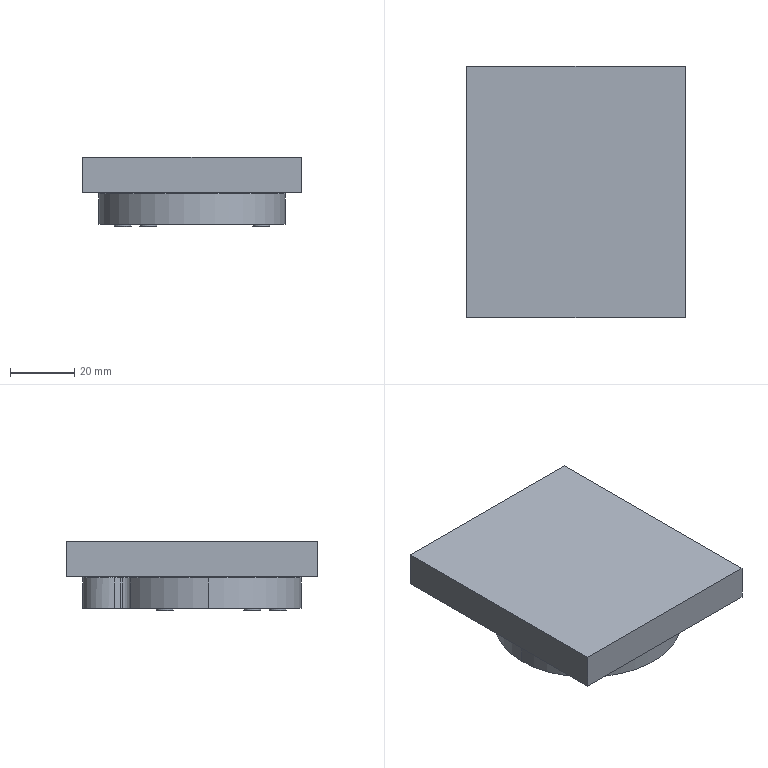NC program | NX | posted with a generic post | part box 68 x 78.27 x 21.8 mm
Lines 1195 to 2039 of 3502:
(ZLEVEL_PROFILE_1 , TOOL : D4)
N2376 T11 M6
N2378 G54
N2380 G17 G0 G90 X-5.374 Y-5.654 S9500 M3
N2382 G43 Z30. H11
N2384 Z1.5
N2386 G94 G1 X-5.297 Y-6.222 Z1.47 F1000.
N2388 X-5.21 Y-6.543 Z1.453
N2390 X-5.125 Y-6.859 Z1.435
N2392 X-4.841 Y-7.546 Z1.396
N2394 X-4.464 Y-8.186 Z1.358
N2396 X-4.003 Y-8.768 Z1.319
N2398 X-3.768 Y-8.996 Z1.301
N2400 X-3.75 Y-9.035 Z1.299
N2402 X3.732 Z0.907
N2404 X3.969 Y-8.808 Z0.89
N2406 X4.539 Y-8.078 Z0.841
N2408 X4.975 Y-7.261 Z0.793
N2410 X5.265 Y-6.382 Z0.744
N2412 X5.4 Y-5.466 Z0.696
N2414 Y-5.137 Z0.679
N2416 Y-4.808 Z0.661
N2418 X5.265 Y-3.892 Z0.613
N2420 X4.976 Y-3.012 Z0.564
N2422 X4.541 Y-2.194 Z0.516
N2424 X3.972 Y-1.462 Z0.467
N2426 X3.735 Y-1.235 Z0.45
N2428 X-3.735 Y-1.236 Z0.058
N2430 X-4.07 Y-1.588 Z0.033
N2432 X-4.287 Y-1.837 Z0.016
N2434 X-4.771 Y-2.589 Z-0.031
N2436 X-5.126 Y-3.411 Z-0.078
N2438 X-5.212 Y-3.729 Z-0.096
N2440 X-5.297 Y-4.047 Z-0.113
N2442 X-5.395 Y-4.77 Z-0.151
N2444 Y-5.499 Z-0.189
N2446 X-5.297 Y-6.222 Z-0.227
N2448 X-5.21 Y-6.543 Z-0.245
N2450 X-5.125 Y-6.859 Z-0.262
N2452 X-4.841 Y-7.546 Z-0.301
N2454 X-4.464 Y-8.186 Z-0.34
N2456 X-4.003 Y-8.768 Z-0.379
N2458 X-3.768 Y-8.996 Z-0.396
N2460 X-3.75 Y-9.035 Z-0.398
N2462 X-3.717 Z-0.4
N2464 X3.732 F2500.
N2466 G3 X5.4 Y-5.137 R5.389
N2468 X3.735 Y-1.235 R5.405
N2470 G1 X-3.735 Y-1.236
N2472 X-4.07 Y-1.588
N2474 G3 X-5.212 Y-3.729 R5.451
N2476 X-5.21 Y-6.543 R5.408
N2478 X-3.768 Y-8.996 R5.347
N2480 G1 X-3.765 Y-9.003
N2482 X-3.76 Y-9.027
N2484 X-3.74 Y-9.04
N2486 X-3.717 Y-9.035
N2488 X0.008 Z-0.446
N2490 X1.87 Z-0.469
N2492 X3.731 Y-9.034 Z-0.492
N2494 X3.79 Y-8.974 Z-0.493
N2496 X4.155 Y-8.579 Z-0.5
N2498 X4.252 Y-8.457 Z-0.502
N2500 X4.348 Y-8.335 Z-0.504
N2502 X4.439 Y-8.209 Z-0.506
N2504 X4.524 Y-8.078 Z-0.507
N2506 X4.609 Y-7.948 Z-0.509
N2508 X4.688 Y-7.814 Z-0.511
N2510 X4.762 Y-7.677 Z-0.513
N2512 X4.835 Y-7.539 Z-0.515
N2514 X4.966 Y-7.257 Z-0.519
N2516 X5.078 Y-6.967 Z-0.523
N2518 X5.129 Y-6.82 Z-0.525
N2520 X5.177 Y-6.672 Z-0.527
N2522 X5.217 Y-6.522 Z-0.529
N2524 X5.254 Y-6.37 Z-0.531
N2526 X5.318 Y-6.066 Z-0.534
N2528 X5.361 Y-5.758 Z-0.538
N2530 X5.385 Y-5.448 Z-0.542
N2532 X5.399 Y-5.137 Z-0.546
N2534 X5.385 Y-4.826 Z-0.55
N2536 X5.362 Y-4.516 Z-0.554
N2538 X5.318 Y-4.208 Z-0.557
N2540 X5.255 Y-3.903 Z-0.561
N2542 X5.218 Y-3.752 Z-0.563
N2544 X5.178 Y-3.601 Z-0.565
N2546 X5.13 Y-3.453 Z-0.567
N2548 X5.079 Y-3.306 Z-0.569
N2550 X5.025 Y-3.16 Z-0.571
N2552 X4.967 Y-3.016 Z-0.573
N2554 X4.902 Y-2.874 Z-0.575
N2556 X4.836 Y-2.733 Z-0.577
N2558 X4.689 Y-2.458 Z-0.581
N2560 X4.526 Y-2.194 Z-0.584
N2562 X4.44 Y-2.063 Z-0.586
N2564 X4.35 Y-1.937 Z-0.588
N2566 X4.253 Y-1.815 Z-0.59
N2568 X4.156 Y-1.693 Z-0.592
N2570 X3.734 Y-1.237 Z-0.6
N2572 X1.867 Y-1.235 Z-0.623
N2574 X0. Z-0.646
N2576 X-1.865 Z-0.669
N2578 X-3.728 Y-1.237 Z-0.692
N2580 X-3.777 Y-1.283 Z-0.693
N2582 X-4.07 Y-1.587 Z-0.698
N2584 X-4.26 Y-1.827 Z-0.702
N2586 X-4.444 Y-2.072 Z-0.706
N2588 X-4.609 Y-2.329 Z-0.709
N2590 X-4.762 Y-2.594 Z-0.713
N2592 X-4.831 Y-2.731 Z-0.715
N2594 X-4.9 Y-2.867 Z-0.717
N2596 X-4.962 Y-3.007 Z-0.719
N2598 X-5.018 Y-3.15 Z-0.721
N2600 X-5.073 Y-3.292 Z-0.723
N2602 X-5.125 Y-3.436 Z-0.725
N2604 X-5.17 Y-3.582 Z-0.727
N2606 X-5.212 Y-3.73 Z-0.728
N2608 X-5.281 Y-4.005 Z-0.732
N2610 X-5.331 Y-4.285 Z-0.735
N2612 X-5.37 Y-4.567 Z-0.739
N2614 X-5.392 Y-4.85 Z-0.742
N2616 X-5.4 Y-5.134 Z-0.746
N2618 X-5.393 Y-5.419 Z-0.749
N2620 X-5.37 Y-5.702 Z-0.753
N2622 X-5.331 Y-5.984 Z-0.757
N2624 X-5.28 Y-6.266 Z-0.76
N2626 X-5.21 Y-6.543 Z-0.764
N2628 X-5.172 Y-6.682 Z-0.765
N2630 X-5.13 Y-6.82 Z-0.767
N2632 X-5.082 Y-6.956 Z-0.769
N2634 X-5.03 Y-7.09 Z-0.771
N2636 X-4.977 Y-7.224 Z-0.772
N2638 X-4.922 Y-7.357 Z-0.774
N2640 X-4.857 Y-7.486 Z-0.776
N2642 X-4.792 Y-7.614 Z-0.778
N2644 X-4.727 Y-7.743 Z-0.78
N2646 X-4.656 Y-7.868 Z-0.781
N2648 X-4.578 Y-7.989 Z-0.783
N2650 X-4.501 Y-8.11 Z-0.785
N2652 X-4.336 Y-8.346 Z-0.789
N2654 X-4.158 Y-8.573 Z-0.792
N2656 X-3.966 Y-8.791 Z-0.796
N2658 X-3.742 Y-9.023 Z-0.8
N2660 X-3.717 Y-9.035
N2662 X0.009 Z-0.846
N2664 X1.871 Z-0.869
N2666 X3.732 Y-9.033 Z-0.892
N2668 X3.76 Y-9.006 Z-0.893
N2670 X3.974 Y-8.785 Z-0.896
N2672 X4.176 Y-8.552 Z-0.9
N2674 X4.272 Y-8.431 Z-0.902
N2676 X4.368 Y-8.31 Z-0.904
N2678 X4.455 Y-8.184 Z-0.906
N2680 X4.54 Y-8.055 Z-0.908
N2682 X4.701 Y-7.792 Z-0.912
N2684 X4.845 Y-7.519 Z-0.915
N2686 X4.973 Y-7.239 Z-0.919
N2688 X5.084 Y-6.951 Z-0.923
N2690 X5.134 Y-6.805 Z-0.925
N2692 X5.181 Y-6.658 Z-0.927
N2694 X5.221 Y-6.509 Z-0.929
N2696 X5.257 Y-6.359 Z-0.931
N2698 X5.318 Y-6.057 Z-0.934
N2700 X5.362 Y-5.752 Z-0.938
N2702 X5.385 Y-5.445 Z-0.942
N2704 X5.399 Y-5.137 Z-0.946
N2706 X5.385 Y-4.826 Z-0.95
N2708 X5.362 Y-4.516 Z-0.954
N2710 X5.318 Y-4.208 Z-0.957
N2712 X5.255 Y-3.903 Z-0.961
N2714 X5.218 Y-3.752 Z-0.963
N2716 X5.178 Y-3.601 Z-0.965
N2718 X5.13 Y-3.453 Z-0.967
N2720 X5.079 Y-3.306 Z-0.969
N2722 X4.967 Y-3.016 Z-0.973
N2724 X4.836 Y-2.733 Z-0.977
N2726 X4.689 Y-2.458 Z-0.981
N2728 X4.526 Y-2.194 Z-0.984
N2730 X4.441 Y-2.063 Z-0.986
N2732 X4.35 Y-1.937 Z-0.988
N2734 X4.253 Y-1.815 Z-0.99
N2736 X4.156 Y-1.693 Z-0.992
N2738 X3.734 Y-1.237 Z-1.
N2740 X1.867 Y-1.235 Z-1.023
N2742 X0. Z-1.046
N2744 X-1.867 Z-1.069
N2746 X-3.734 Y-1.238 Z-1.092
N2748 X-3.791 Y-1.297 Z-1.093
N2750 X-4.155 Y-1.693 Z-1.1
N2752 X-4.347 Y-1.938 Z-1.104
N2754 X-4.523 Y-2.194 Z-1.107
N2756 X-4.607 Y-2.326 Z-1.109
N2758 X-4.689 Y-2.457 Z-1.111
N2760 X-4.761 Y-2.595 Z-1.113
N2762 X-4.833 Y-2.734 Z-1.115
N2764 X-4.965 Y-3.015 Z-1.119
N2766 X-5.079 Y-3.305 Z-1.123
N2768 X-5.174 Y-3.601 Z-1.127
N2770 X-5.257 Y-3.901 Z-1.131
N2772 X-5.317 Y-4.206 Z-1.134
N2774 X-5.363 Y-4.514 Z-1.138
N2776 X-5.39 Y-4.824 Z-1.142
N2778 X-5.4 Y-5.135 Z-1.146
N2780 X-5.39 Y-5.446 Z-1.15
N2782 X-5.363 Y-5.756 Z-1.154
N2784 X-5.317 Y-6.064 Z-1.157
N2786 X-5.257 Y-6.369 Z-1.161
N2788 X-5.174 Y-6.669 Z-1.165
N2790 X-5.079 Y-6.965 Z-1.169
N2792 X-4.965 Y-7.254 Z-1.173
N2794 X-4.833 Y-7.536 Z-1.177
N2796 X-4.761 Y-7.674 Z-1.179
N2798 X-4.689 Y-7.812 Z-1.181
N2800 X-4.607 Y-7.944 Z-1.182
N2802 X-4.523 Y-8.075 Z-1.184
N2804 X-4.347 Y-8.332 Z-1.188
N2806 X-4.155 Y-8.576 Z-1.192
N2808 X-3.786 Y-8.978 Z-1.199
N2810 X-3.734 Y-9.032 Z-1.2
N2812 X-3.717 Y-9.035
N2814 X0.009 Z-1.246
N2816 X1.871 Z-1.269
N2818 X3.732 Y-9.033 Z-1.292
N2820 X3.76 Y-9.006 Z-1.293
N2822 X3.974 Y-8.785 Z-1.296
N2824 X4.176 Y-8.552 Z-1.3
N2826 X4.272 Y-8.431 Z-1.302
N2828 X4.368 Y-8.31 Z-1.304
N2830 X4.455 Y-8.184 Z-1.306
N2832 X4.54 Y-8.055 Z-1.308
N2834 X4.701 Y-7.792 Z-1.312
N2836 X4.845 Y-7.519 Z-1.315
N2838 X4.973 Y-7.239 Z-1.319
N2840 X5.084 Y-6.951 Z-1.323
N2842 X5.134 Y-6.805 Z-1.325
N2844 X5.181 Y-6.658 Z-1.327
N2846 X5.221 Y-6.509 Z-1.329
N2848 X5.257 Y-6.359 Z-1.331
N2850 X5.318 Y-6.057 Z-1.334
N2852 X5.362 Y-5.752 Z-1.338
N2854 X5.385 Y-5.445 Z-1.342
N2856 X5.399 Y-5.137 Z-1.346
N2858 X5.385 Y-4.826 Z-1.35
N2860 X5.362 Y-4.516 Z-1.354
N2862 X5.318 Y-4.208 Z-1.357
N2864 X5.255 Y-3.903 Z-1.361
N2866 X5.218 Y-3.752 Z-1.363
N2868 X5.178 Y-3.601 Z-1.365
N2870 X5.13 Y-3.453 Z-1.367
N2872 X5.079 Y-3.306 Z-1.369
N2874 X4.967 Y-3.016 Z-1.373
N2876 X4.836 Y-2.733 Z-1.377
N2878 X4.689 Y-2.458 Z-1.381
N2880 X4.526 Y-2.194 Z-1.384
N2882 X4.44 Y-2.063 Z-1.386
N2884 X4.35 Y-1.937 Z-1.388
N2886 X4.253 Y-1.815 Z-1.39
N2888 X4.156 Y-1.693 Z-1.392
N2890 X3.734 Y-1.237 Z-1.4
N2892 X1.867 Y-1.235 Z-1.423
N2894 X0. Z-1.446
N2896 X-1.867 Z-1.469
N2898 X-3.734 Y-1.238 Z-1.492
N2900 X-3.791 Y-1.297 Z-1.493
N2902 X-4.155 Y-1.693 Z-1.5
N2904 X-4.347 Y-1.938 Z-1.504
N2906 X-4.523 Y-2.194 Z-1.507
N2908 X-4.607 Y-2.326 Z-1.509
N2910 X-4.689 Y-2.457 Z-1.511
N2912 X-4.761 Y-2.595 Z-1.513
N2914 X-4.833 Y-2.734 Z-1.515
N2916 X-4.965 Y-3.015 Z-1.519
N2918 X-5.079 Y-3.305 Z-1.523
N2920 X-5.174 Y-3.601 Z-1.527
N2922 X-5.257 Y-3.901 Z-1.531
N2924 X-5.317 Y-4.206 Z-1.534
N2926 X-5.363 Y-4.514 Z-1.538
N2928 X-5.39 Y-4.824 Z-1.542
N2930 X-5.4 Y-5.135 Z-1.546
N2932 X-5.39 Y-5.446 Z-1.55
N2934 X-5.363 Y-5.756 Z-1.554
N2936 X-5.317 Y-6.064 Z-1.557
N2938 X-5.257 Y-6.369 Z-1.561
N2940 X-5.174 Y-6.669 Z-1.565
N2942 X-5.079 Y-6.965 Z-1.569
N2944 X-4.965 Y-7.254 Z-1.573
N2946 X-4.833 Y-7.536 Z-1.577
N2948 X-4.761 Y-7.674 Z-1.579
N2950 X-4.689 Y-7.812 Z-1.581
N2952 X-4.607 Y-7.944 Z-1.582
N2954 X-4.523 Y-8.075 Z-1.584
N2956 X-4.347 Y-8.332 Z-1.588
N2958 X-4.155 Y-8.576 Z-1.592
N2960 X-3.786 Y-8.978 Z-1.599
N2962 X-3.734 Y-9.031 Z-1.6
N2964 X-3.717 Y-9.035
N2966 X0.009 Z-1.646
N2968 X1.871 Z-1.669
N2970 X3.732 Y-9.033 Z-1.692
N2972 X3.76 Y-9.006 Z-1.693
N2974 X3.974 Y-8.785 Z-1.696
N2976 X4.176 Y-8.552 Z-1.7
N2978 X4.272 Y-8.431 Z-1.702
N2980 X4.368 Y-8.31 Z-1.704
N2982 X4.455 Y-8.184 Z-1.706
N2984 X4.54 Y-8.055 Z-1.708
N2986 X4.701 Y-7.792 Z-1.712
N2988 X4.845 Y-7.519 Z-1.715
N2990 X4.973 Y-7.239 Z-1.719
N2992 X5.084 Y-6.951 Z-1.723
N2994 X5.134 Y-6.805 Z-1.725
N2996 X5.181 Y-6.658 Z-1.727
N2998 X5.221 Y-6.509 Z-1.729
N3000 X5.257 Y-6.359 Z-1.731
N3002 X5.318 Y-6.057 Z-1.734
N3004 X5.362 Y-5.752 Z-1.738
N3006 X5.385 Y-5.445 Z-1.742
N3008 X5.399 Y-5.137 Z-1.746
N3010 X5.385 Y-4.826 Z-1.75
N3012 X5.362 Y-4.516 Z-1.754
N3014 X5.318 Y-4.208 Z-1.757
N3016 X5.255 Y-3.903 Z-1.761
N3018 X5.218 Y-3.752 Z-1.763
N3020 X5.178 Y-3.601 Z-1.765
N3022 X5.13 Y-3.453 Z-1.767
N3024 X5.079 Y-3.306 Z-1.769
N3026 X4.967 Y-3.016 Z-1.773
N3028 X4.836 Y-2.733 Z-1.777
N3030 X4.689 Y-2.458 Z-1.781
N3032 X4.526 Y-2.194 Z-1.784
N3034 X4.44 Y-2.063 Z-1.786
N3036 X4.35 Y-1.937 Z-1.788
N3038 X4.253 Y-1.815 Z-1.79
N3040 X4.156 Y-1.693 Z-1.792
N3042 X3.734 Y-1.237 Z-1.8
N3044 X1.867 Y-1.235 Z-1.823
N3046 X0. Z-1.846
N3048 X-1.867 Z-1.869
N3050 X-3.734 Y-1.238 Z-1.892
N3052 X-3.791 Y-1.297 Z-1.893
N3054 X-4.155 Y-1.693 Z-1.9
N3056 X-4.347 Y-1.938 Z-1.904
N3058 X-4.523 Y-2.194 Z-1.907
N3060 X-4.607 Y-2.326 Z-1.909
N3062 X-4.689 Y-2.457 Z-1.911
N3064 X-4.761 Y-2.595 Z-1.913
N3066 X-4.833 Y-2.734 Z-1.915
N3068 X-4.965 Y-3.015 Z-1.919
N3070 X-5.079 Y-3.305 Z-1.923
N3072 X-5.174 Y-3.601 Z-1.927
N3074 X-5.257 Y-3.901 Z-1.931
N3076 X-5.317 Y-4.206 Z-1.934
N3078 X-5.363 Y-4.514 Z-1.938
N3080 X-5.39 Y-4.824 Z-1.942
N3082 X-5.4 Y-5.135 Z-1.946
N3084 X-5.39 Y-5.446 Z-1.95
N3086 X-5.363 Y-5.756 Z-1.954
N3088 X-5.317 Y-6.064 Z-1.957
N3090 X-5.257 Y-6.369 Z-1.961
N3092 X-5.174 Y-6.669 Z-1.965
N3094 X-5.079 Y-6.965 Z-1.969
N3096 X-4.965 Y-7.254 Z-1.973
N3098 X-4.833 Y-7.536 Z-1.977
N3100 X-4.761 Y-7.674 Z-1.979
N3102 X-4.689 Y-7.812 Z-1.981
N3104 X-4.607 Y-7.944 Z-1.982
N3106 X-4.523 Y-8.075 Z-1.984
N3108 X-4.347 Y-8.332 Z-1.988
N3110 X-4.155 Y-8.576 Z-1.992
N3112 X-3.786 Y-8.978 Z-1.999
N3114 X-3.734 Y-9.031 Z-2.
N3116 X-3.717 Y-9.035
N3118 X0.009 Z-2.046
N3120 X1.871 Z-2.069
N3122 X3.732 Y-9.033 Z-2.092
N3124 X3.76 Y-9.006 Z-2.093
N3126 X3.974 Y-8.785 Z-2.096
N3128 X4.176 Y-8.552 Z-2.1
N3130 X4.272 Y-8.431 Z-2.102
N3132 X4.368 Y-8.31 Z-2.104
N3134 X4.455 Y-8.184 Z-2.106
N3136 X4.54 Y-8.055 Z-2.108
N3138 X4.701 Y-7.792 Z-2.112
N3140 X4.845 Y-7.519 Z-2.115
N3142 X4.973 Y-7.239 Z-2.119
N3144 X5.084 Y-6.951 Z-2.123
N3146 X5.134 Y-6.805 Z-2.125
N3148 X5.181 Y-6.658 Z-2.127
N3150 X5.221 Y-6.509 Z-2.129
N3152 X5.257 Y-6.359 Z-2.131
N3154 X5.318 Y-6.057 Z-2.134
N3156 X5.362 Y-5.752 Z-2.138
N3158 X5.385 Y-5.445 Z-2.142
N3160 X5.399 Y-5.137 Z-2.146
N3162 X5.385 Y-4.826 Z-2.15
N3164 X5.362 Y-4.516 Z-2.154
N3166 X5.318 Y-4.208 Z-2.157
N3168 X5.255 Y-3.903 Z-2.161
N3170 X5.218 Y-3.752 Z-2.163
N3172 X5.178 Y-3.601 Z-2.165
N3174 X5.13 Y-3.453 Z-2.167
N3176 X5.079 Y-3.306 Z-2.169
N3178 X4.967 Y-3.016 Z-2.173
N3180 X4.836 Y-2.733 Z-2.177
N3182 X4.689 Y-2.459 Z-2.181
N3184 X4.526 Y-2.194 Z-2.184
N3186 X4.44 Y-2.063 Z-2.186
N3188 X4.35 Y-1.937 Z-2.188
N3190 X4.253 Y-1.815 Z-2.19
N3192 X4.156 Y-1.693 Z-2.192
N3194 X3.734 Y-1.237 Z-2.2
N3196 X1.867 Y-1.235 Z-2.223
N3198 X0. Z-2.246
N3200 X-1.867 Z-2.269
N3202 X-3.734 Y-1.238 Z-2.292
N3204 X-3.791 Y-1.297 Z-2.293
N3206 X-4.155 Y-1.693 Z-2.3
N3208 X-4.347 Y-1.938 Z-2.304
N3210 X-4.523 Y-2.194 Z-2.307
N3212 X-4.607 Y-2.326 Z-2.309
N3214 X-4.689 Y-2.457 Z-2.311
N3216 X-4.761 Y-2.595 Z-2.313
N3218 X-4.833 Y-2.734 Z-2.315
N3220 X-4.965 Y-3.015 Z-2.319
N3222 X-5.079 Y-3.305 Z-2.323
N3224 X-5.174 Y-3.601 Z-2.327
N3226 X-5.257 Y-3.901 Z-2.331
N3228 X-5.317 Y-4.206 Z-2.334
N3230 X-5.363 Y-4.514 Z-2.338
N3232 X-5.39 Y-4.824 Z-2.342
N3234 X-5.4 Y-5.135 Z-2.346
N3236 X-5.39 Y-5.446 Z-2.35
N3238 X-5.363 Y-5.756 Z-2.354
N3240 X-5.317 Y-6.064 Z-2.357
N3242 X-5.257 Y-6.369 Z-2.361
N3244 X-5.174 Y-6.669 Z-2.365
N3246 X-5.079 Y-6.965 Z-2.369
N3248 X-4.965 Y-7.254 Z-2.373
N3250 X-4.833 Y-7.536 Z-2.377
N3252 X-4.761 Y-7.674 Z-2.379
N3254 X-4.689 Y-7.812 Z-2.381
N3256 X-4.607 Y-7.944 Z-2.382
N3258 X-4.523 Y-8.075 Z-2.384
N3260 X-4.347 Y-8.332 Z-2.388
N3262 X-4.155 Y-8.576 Z-2.392
N3264 X-3.786 Y-8.978 Z-2.399
N3266 X-3.734 Y-9.031 Z-2.4
N3268 X-3.717 Y-9.035
N3270 X0.009 Z-2.446
N3272 X1.871 Z-2.469
N3274 X3.732 Y-9.033 Z-2.492
N3276 X3.76 Y-9.006 Z-2.493
N3278 X3.974 Y-8.785 Z-2.496
N3280 X4.176 Y-8.552 Z-2.5
N3282 X4.272 Y-8.431 Z-2.502
N3284 X4.368 Y-8.31 Z-2.504
N3286 X4.455 Y-8.184 Z-2.506
N3288 X4.54 Y-8.054 Z-2.508
N3290 X4.701 Y-7.792 Z-2.512
N3292 X4.845 Y-7.519 Z-2.515
N3294 X4.973 Y-7.239 Z-2.519
N3296 X5.084 Y-6.951 Z-2.523
N3298 X5.134 Y-6.805 Z-2.525
N3300 X5.181 Y-6.658 Z-2.527
N3302 X5.221 Y-6.509 Z-2.529
N3304 X5.257 Y-6.359 Z-2.531
N3306 X5.318 Y-6.057 Z-2.534
N3308 X5.362 Y-5.752 Z-2.538
N3310 X5.385 Y-5.445 Z-2.542
N3312 X5.399 Y-5.137 Z-2.546
N3314 X5.385 Y-4.826 Z-2.55
N3316 X5.362 Y-4.516 Z-2.554
N3318 X5.318 Y-4.208 Z-2.557
N3320 X5.255 Y-3.903 Z-2.561
N3322 X5.218 Y-3.752 Z-2.563
N3324 X5.178 Y-3.601 Z-2.565
N3326 X5.13 Y-3.453 Z-2.567
N3328 X5.079 Y-3.306 Z-2.569
N3330 X4.967 Y-3.016 Z-2.573
N3332 X4.836 Y-2.733 Z-2.577
N3334 X4.689 Y-2.458 Z-2.581
N3336 X4.526 Y-2.194 Z-2.584
N3338 X4.44 Y-2.063 Z-2.586
N3340 X4.35 Y-1.937 Z-2.588
N3342 X4.253 Y-1.815 Z-2.59
N3344 X4.156 Y-1.693 Z-2.592
N3346 X3.734 Y-1.237 Z-2.6
N3348 X1.867 Y-1.235 Z-2.623
N3350 X0. Z-2.646
N3352 X-1.867 Z-2.669
N3354 X-3.734 Y-1.238 Z-2.692
N3356 X-3.791 Y-1.297 Z-2.693
N3358 X-4.155 Y-1.693 Z-2.7
N3360 X-4.347 Y-1.938 Z-2.704
N3362 X-4.523 Y-2.194 Z-2.707
N3364 X-4.607 Y-2.326 Z-2.709
N3366 X-4.689 Y-2.457 Z-2.711
N3368 X-4.761 Y-2.595 Z-2.713
N3370 X-4.833 Y-2.734 Z-2.715
N3372 X-4.965 Y-3.015 Z-2.719
N3374 X-5.079 Y-3.305 Z-2.723
N3376 X-5.174 Y-3.601 Z-2.727
N3378 X-5.257 Y-3.901 Z-2.731
N3380 X-5.317 Y-4.206 Z-2.734
N3382 X-5.363 Y-4.514 Z-2.738
N3384 X-5.39 Y-4.824 Z-2.742
N3386 X-5.4 Y-5.135 Z-2.746
N3388 X-5.39 Y-5.446 Z-2.75
N3390 X-5.363 Y-5.756 Z-2.754
N3392 X-5.317 Y-6.064 Z-2.757
N3394 X-5.257 Y-6.369 Z-2.761
N3396 X-5.174 Y-6.669 Z-2.765
N3398 X-5.079 Y-6.965 Z-2.769
N3400 X-4.965 Y-7.254 Z-2.773
N3402 X-4.833 Y-7.536 Z-2.777
N3404 X-4.761 Y-7.674 Z-2.779
N3406 X-4.689 Y-7.812 Z-2.781
N3408 X-4.607 Y-7.944 Z-2.782
N3410 X-4.523 Y-8.075 Z-2.784
N3412 X-4.347 Y-8.332 Z-2.788
N3414 X-4.155 Y-8.576 Z-2.792
N3416 X-3.786 Y-8.978 Z-2.799
N3418 X-3.734 Y-9.031 Z-2.8
N3420 X-3.717 Y-9.035
N3422 X0.009 Z-2.846
N3424 X1.871 Z-2.869
N3426 X3.732 Y-9.033 Z-2.892
N3428 X3.76 Y-9.006 Z-2.893
N3430 X3.974 Y-8.785 Z-2.896
N3432 X4.176 Y-8.552 Z-2.9
N3434 X4.272 Y-8.431 Z-2.902
N3436 X4.368 Y-8.31 Z-2.904
N3438 X4.455 Y-8.184 Z-2.906
N3440 X4.54 Y-8.054 Z-2.908
N3442 X4.701 Y-7.792 Z-2.912
N3444 X4.845 Y-7.519 Z-2.915
N3446 X4.973 Y-7.239 Z-2.919
N3448 X5.084 Y-6.951 Z-2.923
N3450 X5.134 Y-6.805 Z-2.925
N3452 X5.181 Y-6.658 Z-2.927
N3454 X5.221 Y-6.509 Z-2.929
N3456 X5.257 Y-6.359 Z-2.931
N3458 X5.318 Y-6.057 Z-2.934
N3460 X5.362 Y-5.752 Z-2.938
N3462 X5.385 Y-5.445 Z-2.942
N3464 X5.399 Y-5.137 Z-2.946
N3466 X5.385 Y-4.826 Z-2.95
N3468 X5.362 Y-4.516 Z-2.954
N3470 X5.318 Y-4.208 Z-2.957
N3472 X5.255 Y-3.903 Z-2.961
N3474 X5.218 Y-3.752 Z-2.963
N3476 X5.178 Y-3.601 Z-2.965
N3478 X5.13 Y-3.453 Z-2.967
N3480 X5.079 Y-3.306 Z-2.969
N3482 X4.967 Y-3.016 Z-2.973
N3484 X4.836 Y-2.733 Z-2.977
N3486 X4.689 Y-2.458 Z-2.981
N3488 X4.526 Y-2.194 Z-2.984
N3490 X4.44 Y-2.063 Z-2.986
N3492 X4.35 Y-1.937 Z-2.988
N3494 X4.253 Y-1.815 Z-2.99
N3496 X4.156 Y-1.693 Z-2.992
N3498 X3.734 Y-1.237 Z-3.
N3500 X1.867 Y-1.235 Z-3.023
N3502 X0. Z-3.046
N3504 X-1.867 Z-3.069
N3506 X-3.734 Y-1.238 Z-3.092
N3508 X-3.791 Y-1.297 Z-3.093
N3510 X-4.155 Y-1.693 Z-3.1
N3512 X-4.347 Y-1.938 Z-3.104
N3514 X-4.523 Y-2.194 Z-3.107
N3516 X-4.607 Y-2.326 Z-3.109
N3518 X-4.689 Y-2.457 Z-3.111
N3520 X-4.761 Y-2.595 Z-3.113
N3522 X-4.833 Y-2.734 Z-3.115
N3524 X-4.965 Y-3.015 Z-3.119
N3526 X-5.079 Y-3.305 Z-3.123
N3528 X-5.174 Y-3.601 Z-3.127
N3530 X-5.257 Y-3.901 Z-3.131
N3532 X-5.317 Y-4.206 Z-3.134
N3534 X-5.363 Y-4.514 Z-3.138
N3536 X-5.39 Y-4.824 Z-3.142
N3538 X-5.4 Y-5.135 Z-3.146
N3540 X-5.39 Y-5.446 Z-3.15
N3542 X-5.363 Y-5.756 Z-3.154
N3544 X-5.317 Y-6.064 Z-3.157
N3546 X-5.257 Y-6.369 Z-3.161
N3548 X-5.174 Y-6.669 Z-3.165
N3550 X-5.079 Y-6.965 Z-3.169
N3552 X-4.965 Y-7.254 Z-3.173
N3554 X-4.833 Y-7.536 Z-3.177
N3556 X-4.761 Y-7.674 Z-3.179
N3558 X-4.689 Y-7.812 Z-3.181
N3560 X-4.607 Y-7.944 Z-3.182
N3562 X-4.523 Y-8.075 Z-3.184
N3564 X-4.347 Y-8.332 Z-3.188
N3566 X-4.155 Y-8.576 Z-3.192
N3568 X-3.786 Y-8.978 Z-3.199
N3570 X-3.734 Y-9.031 Z-3.2
N3572 X-3.717 Y-9.035
N3574 X0.009 Z-3.246
N3576 X1.871 Z-3.269
N3578 X3.732 Y-9.033 Z-3.292
N3580 X3.76 Y-9.006 Z-3.293
N3582 X3.974 Y-8.785 Z-3.296
N3584 X4.176 Y-8.552 Z-3.3
N3586 X4.272 Y-8.431 Z-3.302
N3588 X4.368 Y-8.31 Z-3.304
N3590 X4.455 Y-8.184 Z-3.306
N3592 X4.54 Y-8.054 Z-3.308
N3594 X4.701 Y-7.792 Z-3.312
N3596 X4.845 Y-7.519 Z-3.315
N3598 X4.973 Y-7.239 Z-3.319
N3600 X5.084 Y-6.951 Z-3.323
N3602 X5.134 Y-6.805 Z-3.325
N3604 X5.181 Y-6.658 Z-3.327
N3606 X5.221 Y-6.509 Z-3.329
N3608 X5.257 Y-6.359 Z-3.331
N3610 X5.318 Y-6.057 Z-3.334
N3612 X5.362 Y-5.752 Z-3.338
N3614 X5.385 Y-5.445 Z-3.342
N3616 X5.399 Y-5.137 Z-3.346
N3618 X5.385 Y-4.826 Z-3.35
N3620 X5.362 Y-4.516 Z-3.354
N3622 X5.318 Y-4.208 Z-3.357
N3624 X5.255 Y-3.903 Z-3.361
N3626 X5.218 Y-3.752 Z-3.363
N3628 X5.178 Y-3.601 Z-3.365
N3630 X5.13 Y-3.453 Z-3.367
N3632 X5.079 Y-3.306 Z-3.369
N3634 X4.967 Y-3.016 Z-3.373
N3636 X4.836 Y-2.733 Z-3.377
N3638 X4.689 Y-2.459 Z-3.381
N3640 X4.526 Y-2.194 Z-3.384
N3642 X4.44 Y-2.063 Z-3.386
N3644 X4.35 Y-1.937 Z-3.388
N3646 X4.253 Y-1.815 Z-3.39
N3648 X4.156 Y-1.693 Z-3.392
N3650 X3.734 Y-1.237 Z-3.4
N3652 X1.867 Y-1.235 Z-3.423
N3654 X0. Z-3.446
N3656 X-1.867 Z-3.469
N3658 X-3.734 Y-1.238 Z-3.492
N3660 X-3.791 Y-1.297 Z-3.493
N3662 X-4.155 Y-1.693 Z-3.5
N3664 X-4.347 Y-1.938 Z-3.504
N3666 X-4.523 Y-2.194 Z-3.507
N3668 X-4.607 Y-2.326 Z-3.509
N3670 X-4.689 Y-2.457 Z-3.511
N3672 X-4.761 Y-2.595 Z-3.513
N3674 X-4.833 Y-2.734 Z-3.515
N3676 X-4.965 Y-3.015 Z-3.519
N3678 X-5.079 Y-3.305 Z-3.523
N3680 X-5.174 Y-3.601 Z-3.527
N3682 X-5.257 Y-3.901 Z-3.531
N3684 X-5.317 Y-4.206 Z-3.534
N3686 X-5.363 Y-4.514 Z-3.538
N3688 X-5.39 Y-4.824 Z-3.542
N3690 X-5.4 Y-5.135 Z-3.546
N3692 X-5.39 Y-5.446 Z-3.55
N3694 X-5.363 Y-5.756 Z-3.554
N3696 X-5.317 Y-6.064 Z-3.557
N3698 X-5.257 Y-6.369 Z-3.561
N3700 X-5.174 Y-6.669 Z-3.565
N3702 X-5.079 Y-6.965 Z-3.569
N3704 X-4.965 Y-7.254 Z-3.573
N3706 X-4.833 Y-7.536 Z-3.577
N3708 X-4.761 Y-7.674 Z-3.579
N3710 X-4.689 Y-7.812 Z-3.581
N3712 X-4.607 Y-7.944 Z-3.582
N3714 X-4.523 Y-8.075 Z-3.584
N3716 X-4.347 Y-8.332 Z-3.588
N3718 X-4.155 Y-8.576 Z-3.592
N3720 X-3.786 Y-8.978 Z-3.599
N3722 X-3.734 Y-9.031 Z-3.6
N3724 X-3.717 Y-9.035
N3726 X0.009 Z-3.646
N3728 X1.871 Z-3.669
N3730 X3.732 Y-9.033 Z-3.692
N3732 X3.76 Y-9.006 Z-3.693
N3734 X3.974 Y-8.785 Z-3.696
N3736 X4.176 Y-8.552 Z-3.7
N3738 X4.272 Y-8.431 Z-3.702
N3740 X4.368 Y-8.31 Z-3.704
N3742 X4.455 Y-8.184 Z-3.706
N3744 X4.54 Y-8.054 Z-3.708
N3746 X4.701 Y-7.792 Z-3.712
N3748 X4.845 Y-7.519 Z-3.715
N3750 X4.973 Y-7.239 Z-3.719
N3752 X5.084 Y-6.951 Z-3.723
N3754 X5.134 Y-6.805 Z-3.725
N3756 X5.181 Y-6.658 Z-3.727
N3758 X5.221 Y-6.509 Z-3.729
N3760 X5.257 Y-6.359 Z-3.731
N3762 X5.318 Y-6.057 Z-3.734
N3764 X5.362 Y-5.752 Z-3.738
N3766 X5.385 Y-5.445 Z-3.742
N3768 X5.399 Y-5.137 Z-3.746
N3770 X5.385 Y-4.826 Z-3.75
N3772 X5.362 Y-4.516 Z-3.754
N3774 X5.318 Y-4.208 Z-3.757
N3776 X5.255 Y-3.903 Z-3.761
N3778 X5.218 Y-3.752 Z-3.763
N3780 X5.178 Y-3.601 Z-3.765
N3782 X5.13 Y-3.453 Z-3.767
N3784 X5.079 Y-3.306 Z-3.769
N3786 X4.967 Y-3.016 Z-3.773
N3788 X4.836 Y-2.733 Z-3.777
N3790 X4.689 Y-2.458 Z-3.781
N3792 X4.526 Y-2.194 Z-3.784
N3794 X4.44 Y-2.063 Z-3.786
N3796 X4.35 Y-1.937 Z-3.788
N3798 X4.253 Y-1.815 Z-3.79
N3800 X4.156 Y-1.693 Z-3.792
N3802 X3.734 Y-1.237 Z-3.8
N3804 X1.867 Y-1.235 Z-3.823
N3806 X0. Z-3.846
N3808 X-1.867 Z-3.869
N3810 X-3.734 Y-1.238 Z-3.892
N3812 X-3.791 Y-1.297 Z-3.893
N3814 X-4.155 Y-1.693 Z-3.9
N3816 X-4.347 Y-1.938 Z-3.904
N3818 X-4.523 Y-2.194 Z-3.907
N3820 X-4.607 Y-2.326 Z-3.909
N3822 X-4.689 Y-2.457 Z-3.911
N3824 X-4.761 Y-2.595 Z-3.913
N3826 X-4.833 Y-2.734 Z-3.915
N3828 X-4.965 Y-3.015 Z-3.919
N3830 X-5.079 Y-3.305 Z-3.923
N3832 X-5.174 Y-3.601 Z-3.927
N3834 X-5.257 Y-3.901 Z-3.931
N3836 X-5.317 Y-4.206 Z-3.934
N3838 X-5.363 Y-4.514 Z-3.938
N3840 X-5.39 Y-4.824 Z-3.942
N3842 X-5.4 Y-5.135 Z-3.946
N3844 X-5.39 Y-5.446 Z-3.95
N3846 X-5.363 Y-5.756 Z-3.954
N3848 X-5.317 Y-6.064 Z-3.957
N3850 X-5.257 Y-6.369 Z-3.961
N3852 X-5.174 Y-6.669 Z-3.965
N3854 X-5.079 Y-6.965 Z-3.969
N3856 X-4.965 Y-7.254 Z-3.973
N3858 X-4.833 Y-7.536 Z-3.977
N3860 X-4.761 Y-7.674 Z-3.979
N3862 X-4.689 Y-7.812 Z-3.981
N3864 X-4.607 Y-7.944 Z-3.982
N3866 X-4.523 Y-8.075 Z-3.984
N3868 X-4.347 Y-8.332 Z-3.988
N3870 X-4.155 Y-8.576 Z-3.992
N3872 X-3.786 Y-8.978 Z-3.999
N3874 X-3.734 Y-9.031 Z-4.
N3876 X-3.717 Y-9.035
N3878 X0.009 Z-4.046
N3880 X1.871 Z-4.069
N3882 X3.732 Y-9.033 Z-4.092
N3884 X3.76 Y-9.006 Z-4.093
N3886 X3.974 Y-8.785 Z-4.096
N3888 X4.176 Y-8.552 Z-4.1
N3890 X4.272 Y-8.431 Z-4.102
N3892 X4.368 Y-8.31 Z-4.104
N3894 X4.455 Y-8.184 Z-4.106
N3896 X4.54 Y-8.054 Z-4.108
N3898 X4.701 Y-7.792 Z-4.112
N3900 X4.845 Y-7.519 Z-4.115
N3902 X4.973 Y-7.239 Z-4.119
N3904 X5.084 Y-6.951 Z-4.123
N3906 X5.134 Y-6.805 Z-4.125
N3908 X5.181 Y-6.658 Z-4.127
N3910 X5.221 Y-6.509 Z-4.129
N3912 X5.257 Y-6.359 Z-4.131
N3914 X5.318 Y-6.057 Z-4.134
N3916 X5.362 Y-5.752 Z-4.138
N3918 X5.385 Y-5.445 Z-4.142
N3920 X5.399 Y-5.137 Z-4.146
N3922 X5.385 Y-4.826 Z-4.15
N3924 X5.362 Y-4.516 Z-4.154
N3926 X5.318 Y-4.208 Z-4.157
N3928 X5.255 Y-3.903 Z-4.161
N3930 X5.218 Y-3.752 Z-4.163
N3932 X5.178 Y-3.601 Z-4.165
N3934 X5.13 Y-3.453 Z-4.167
N3936 X5.079 Y-3.306 Z-4.169
N3938 X4.967 Y-3.016 Z-4.173
N3940 X4.836 Y-2.733 Z-4.177
N3942 X4.689 Y-2.458 Z-4.181
N3944 X4.526 Y-2.194 Z-4.184
N3946 X4.44 Y-2.063 Z-4.186
N3948 X4.35 Y-1.937 Z-4.188
N3950 X4.253 Y-1.815 Z-4.19
N3952 X4.156 Y-1.693 Z-4.192
N3954 X3.734 Y-1.237 Z-4.2
N3956 X1.867 Y-1.235 Z-4.223
N3958 X0. Z-4.246
N3960 X-1.867 Z-4.269
N3962 X-3.734 Y-1.238 Z-4.292
N3964 X-3.791 Y-1.297 Z-4.293
N3966 X-4.155 Y-1.693 Z-4.3
N3968 X-4.347 Y-1.938 Z-4.304
N3970 X-4.523 Y-2.194 Z-4.307
N3972 X-4.607 Y-2.326 Z-4.309
N3974 X-4.689 Y-2.457 Z-4.311
N3976 X-4.761 Y-2.595 Z-4.313
N3978 X-4.833 Y-2.734 Z-4.315
N3980 X-4.965 Y-3.015 Z-4.319
N3982 X-5.079 Y-3.305 Z-4.323
N3984 X-5.174 Y-3.601 Z-4.327
N3986 X-5.257 Y-3.901 Z-4.331
N3988 X-5.317 Y-4.206 Z-4.334
N3990 X-5.363 Y-4.514 Z-4.338
N3992 X-5.39 Y-4.824 Z-4.342
N3994 X-5.4 Y-5.135 Z-4.346
N3996 X-5.39 Y-5.446 Z-4.35
N3998 X-5.363 Y-5.756 Z-4.354
N4000 X-5.317 Y-6.064 Z-4.357
N4002 X-5.257 Y-6.369 Z-4.361
N4004 X-5.174 Y-6.669 Z-4.365
N4006 X-5.079 Y-6.965 Z-4.369
N4008 X-4.965 Y-7.254 Z-4.373
N4010 X-4.833 Y-7.536 Z-4.377
N4012 X-4.761 Y-7.674 Z-4.379
N4014 X-4.689 Y-7.812 Z-4.381
N4016 X-4.607 Y-7.944 Z-4.382
N4018 X-4.523 Y-8.075 Z-4.384
N4020 X-4.347 Y-8.332 Z-4.388
N4022 X-4.155 Y-8.576 Z-4.392
N4024 X-3.786 Y-8.978 Z-4.399
N4026 X-3.734 Y-9.031 Z-4.4
N4028 X-3.717 Y-9.035
N4030 X0.009 Z-4.446
N4032 X1.871 Z-4.469
N4034 X3.732 Y-9.033 Z-4.492
N4036 X3.76 Y-9.006 Z-4.493
N4038 X3.974 Y-8.785 Z-4.496
N4040 X4.176 Y-8.552 Z-4.5
N4042 X4.272 Y-8.431 Z-4.502
N4044 X4.368 Y-8.31 Z-4.504
N4046 X4.455 Y-8.184 Z-4.506
N4048 X4.54 Y-8.054 Z-4.508
N4050 X4.701 Y-7.791 Z-4.512
N4052 X4.845 Y-7.519 Z-4.515
N4054 X4.973 Y-7.239 Z-4.519
N4056 X5.084 Y-6.951 Z-4.523
N4058 X5.134 Y-6.805 Z-4.525